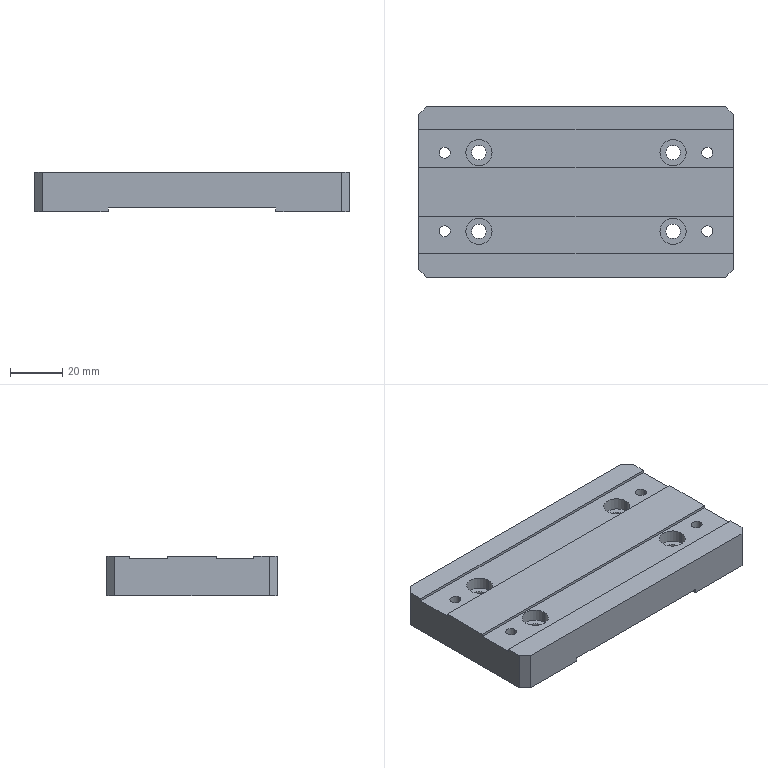Part | STEP file | PN_0016 | 1 solid | 64 faces | box 120 x 65 x 15 mm | volume 102204 mm3 | plane 34 | cylinder 30 | commonest cylinder face diameters 4.2 x8 5.5 x8 10 x8 4 x6